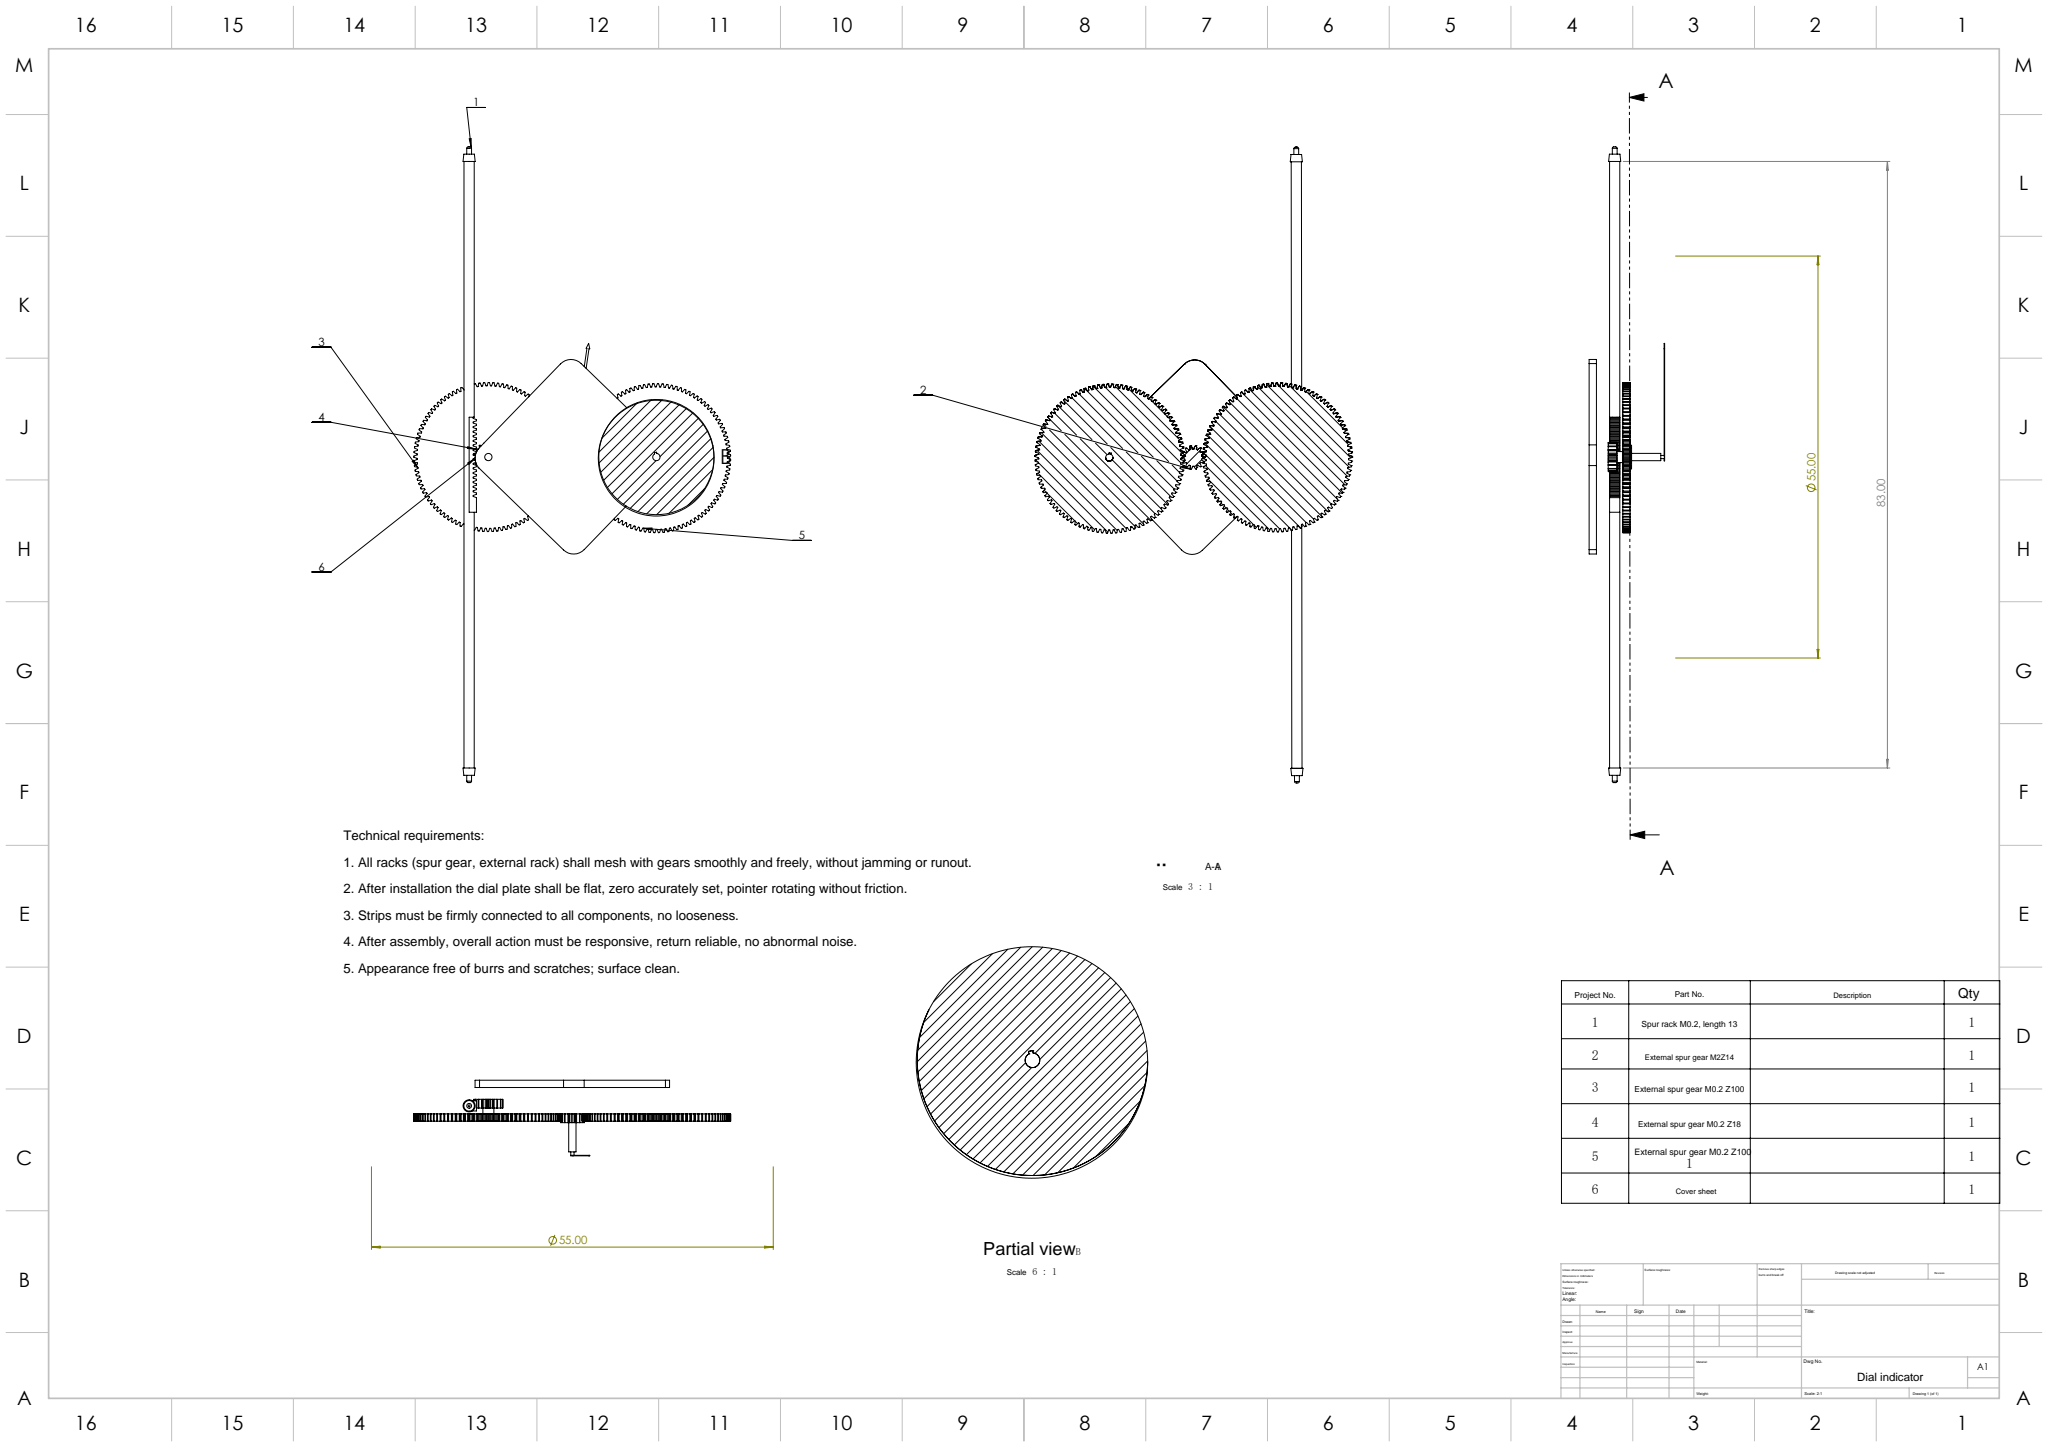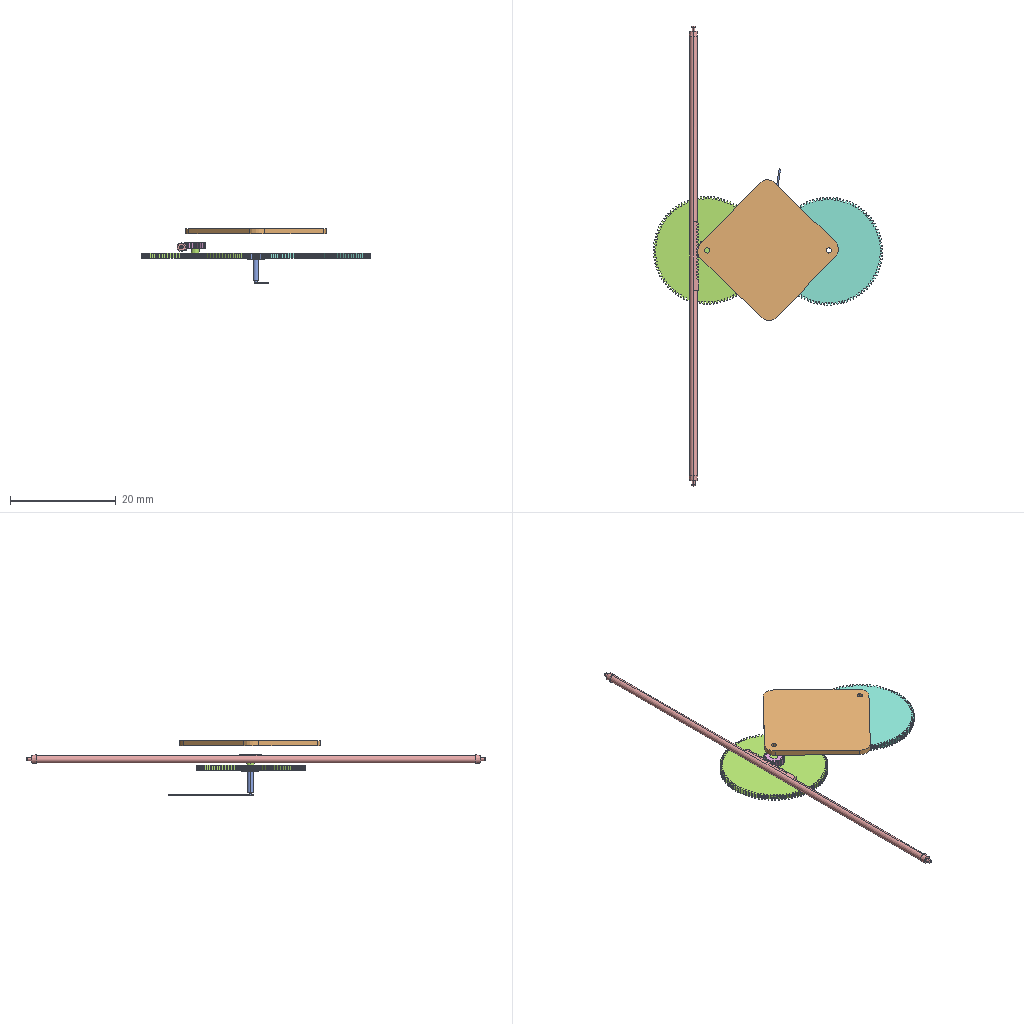Assembly | SolidWorks | 10 different items | 10 placed | box 43 x 87 x 10 mm
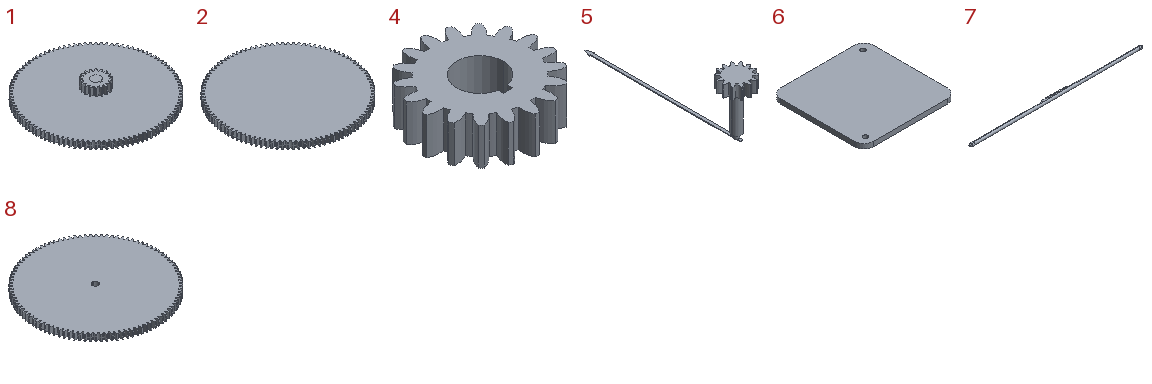Parts list (item | name | quantity | parent item | size | volume | features):
1 | (subassembly) | x1 | - | 20.395 x 20.395 x 3 mm | 326.572 mm3 | -
2 | - | x1 | in 1 | 20.395 x 20.395 x 3 mm | 316.823 mm3 | features ICE 2, CirPattern 1, Extrusion 1
3 | - | x1 | - | - | - | -
4 | - | x1 | in 1 | 3.991 x 3.997 x 1.2 mm | 9.749 mm3 | features ICE 2, CirPattern 1, Extrusion 1
5 | - | x1 | - | 3.258 x 17.347 x 5.736 mm | 10.917 mm3 | features ICE 5, CirPattern 1, Extrusion 1
6 | - | x1 | - | 20 x 20 x 1 mm | 394.996 mm3 | features Extrusion 1, Fillet 1, ICE 1
7 | - | x1 | - | 87 x 1.829 x 1.659 mm | 137.092 mm3 | features ICE 6, Extrusion 1, Fillet 1, LPattern 1, MirrorPattern 1
8 | - | x1 | - | 20.395 x 20.395 x 1 mm | 312.456 mm3 | features ICE 3, CirPattern 1, Extrusion 1
9 | Hairspring | x1 | - | - | - | -
10 | Dial | x1 | - | - | - | -
Mates (type | each side: item.copy, entity, surface, feature):
In the top assembly
Coincident | 5.1 face plane Boss-Extrude1 | 2.1 face plane Boss-Extrude1 | 2 times
GearDim | 5.1 face cylinder CirPattern1 | 2.1 face cylinder Boss-Extrude1
RackPinionDim | 7.1 edge | 4.1 face cylinder Boss-Extrude1
GearDim | 8.1 face cylinder CirPattern1 | 5.1 face cylinder Boss-Extrude1
Coincident | 5.1 face plane Boss-Extrude1 | 8.1 face plane Boss-Extrude1
In subassembly 1
Concentric | 2.2 face cylinder Boss-Extrude3 | 1.1 face
Coincident | 2.2 face plane Boss-Extrude3 | 1.1 face
Concentric | 2.2 face cylinder Boss-Extrude3 | 4.2 face cylinder Boss-Extrude1
Coincident | 2.2 face plane Boss-Extrude3 | 4.2 face plane Boss-Extrude1